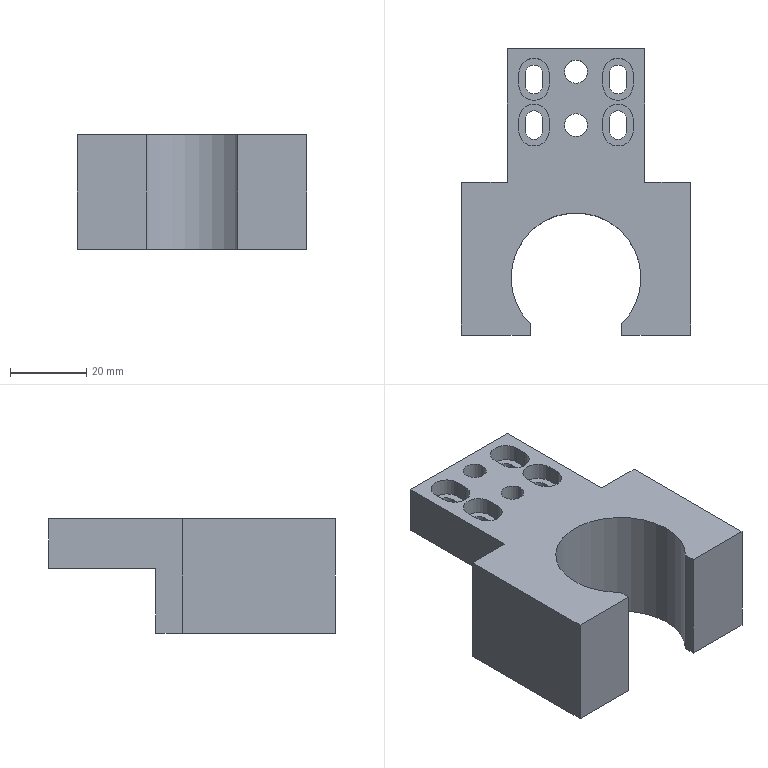Part | NX | features BREP 1 | 1 solid | 74 faces | box 60 x 75 x 30 mm | volume 61974 mm3 | plane 35 | cylinder 31 | cone 8 | commonest cylinder face diameters 4.2 x8 4.5 x8 8 x8 6 x4 34 x3